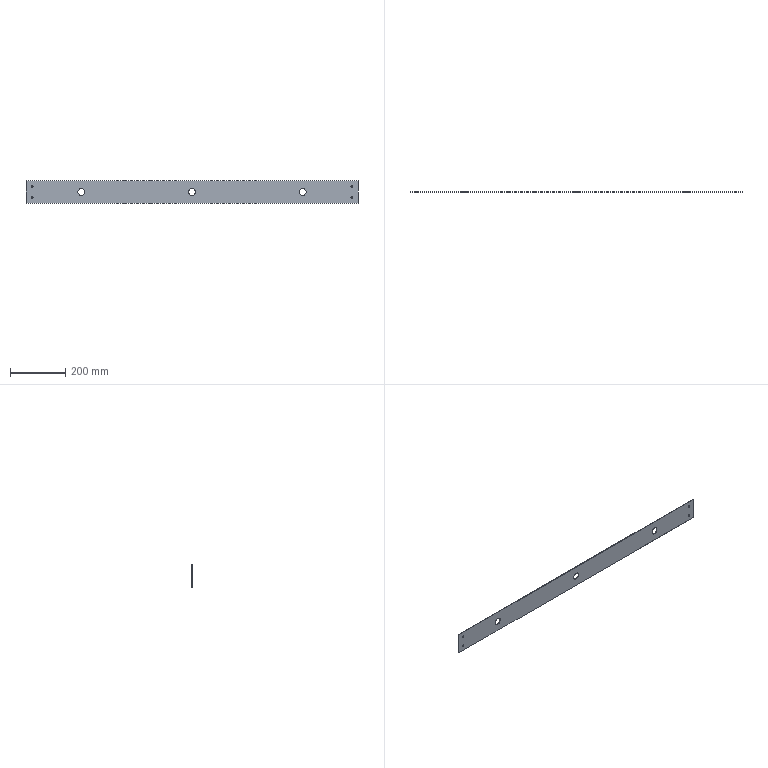Part | SolidWorks | features Extrusion 1 | 1 solid | 20 faces | box 1200 x 2 x 80 mm | volume 188829 mm3 | cylinder 14 | plane 6 | commonest cylinder face diameters 6 x8 25 x6
STEP:
#1=CARTESIAN_POINT('',(0.,2.,-12.5));
#2=VERTEX_POINT('',#1);
#3=CARTESIAN_POINT('',(0.,2.,12.5));
#4=VERTEX_POINT('',#3);
#5=CARTESIAN_POINT('',(0.,2.,0.));
#6=DIRECTION('',(0.,1.,0.));
#7=DIRECTION('',(0.,0.,1.));
#8=AXIS2_PLACEMENT_3D('',#5,#6,#7);
#9=CIRCLE('',#8,12.5);
#10=EDGE_CURVE('',#2,#4,#9,.T.);
#11=ORIENTED_EDGE('',*,*,#10,.T.);
#12=CARTESIAN_POINT('',(0.,0.,12.5));
#13=VERTEX_POINT('',#12);
#14=CARTESIAN_POINT('',(0.,2.,12.5));
#15=DIRECTION('',(0.,-1.,0.));
#16=VECTOR('',#15,1000.);
#17=LINE('',#14,#16);
#18=EDGE_CURVE('',#4,#13,#17,.T.);
#19=ORIENTED_EDGE('',*,*,#18,.T.);
#20=CARTESIAN_POINT('',(0.,0.,-12.5));
#21=VERTEX_POINT('',#20);
#22=CARTESIAN_POINT('',(0.,0.,0.));
#23=DIRECTION('',(0.,1.,0.));
#24=DIRECTION('',(0.,0.,1.));
#25=AXIS2_PLACEMENT_3D('',#22,#23,#24);
#26=CIRCLE('',#25,12.5);
#27=EDGE_CURVE('',#21,#13,#26,.T.);
#28=ORIENTED_EDGE('',*,*,#27,.F.);
#29=CARTESIAN_POINT('',(0.,2.,-12.5));
#30=DIRECTION('',(0.,-1.,0.));
#31=VECTOR('',#30,1000.);
#32=LINE('',#29,#31);
#33=EDGE_CURVE('',#2,#21,#32,.T.);
#34=ORIENTED_EDGE('',*,*,#33,.F.);
#35=EDGE_LOOP('',(#11,#19,#28,#34));
#36=FACE_OUTER_BOUND('',#35,.T.);
#37=CARTESIAN_POINT('',(0.,2.,0.));
#38=DIRECTION('',(0.,-1.,0.));
#39=DIRECTION('',(0.,0.,-1.));
#40=AXIS2_PLACEMENT_3D('',#37,#38,#39);
#41=CYLINDRICAL_SURFACE('',#40,12.5);
#42=ADVANCED_FACE('',(#36),#41,.F.);
#43=CARTESIAN_POINT('',(577.5,2.,17.));
#44=VERTEX_POINT('',#43);
#45=CARTESIAN_POINT('',(577.5,2.,23.));
#46=VERTEX_POINT('',#45);
#47=CARTESIAN_POINT('',(577.5,2.,20.));
#48=DIRECTION('',(0.,1.,0.));
#49=DIRECTION('',(0.,0.,1.));
#50=AXIS2_PLACEMENT_3D('',#47,#48,#49);
#51=CIRCLE('',#50,3.);
#52=EDGE_CURVE('',#44,#46,#51,.T.);
#53=ORIENTED_EDGE('',*,*,#52,.T.);
#54=CARTESIAN_POINT('',(577.5,0.,23.));
#55=VERTEX_POINT('',#54);
#56=CARTESIAN_POINT('',(577.5,2.,23.));
#57=DIRECTION('',(0.,-1.,0.));
#58=VECTOR('',#57,1000.);
#59=LINE('',#56,#58);
#60=EDGE_CURVE('',#46,#55,#59,.T.);
#61=ORIENTED_EDGE('',*,*,#60,.T.);
#62=CARTESIAN_POINT('',(577.5,0.,17.));
#63=VERTEX_POINT('',#62);
#64=CARTESIAN_POINT('',(577.5,0.,20.));
#65=DIRECTION('',(0.,1.,0.));
#66=DIRECTION('',(0.,0.,1.));
#67=AXIS2_PLACEMENT_3D('',#64,#65,#66);
#68=CIRCLE('',#67,3.);
#69=EDGE_CURVE('',#63,#55,#68,.T.);
#70=ORIENTED_EDGE('',*,*,#69,.F.);
#71=CARTESIAN_POINT('',(577.5,2.,17.));
#72=DIRECTION('',(0.,-1.,0.));
#73=VECTOR('',#72,1000.);
#74=LINE('',#71,#73);
#75=EDGE_CURVE('',#44,#63,#74,.T.);
#76=ORIENTED_EDGE('',*,*,#75,.F.);
#77=EDGE_LOOP('',(#53,#61,#70,#76));
#78=FACE_OUTER_BOUND('',#77,.T.);
#79=CARTESIAN_POINT('',(577.5,2.,20.));
#80=DIRECTION('',(0.,-1.,0.));
#81=DIRECTION('',(0.,0.,-1.));
#82=AXIS2_PLACEMENT_3D('',#79,#80,#81);
#83=CYLINDRICAL_SURFACE('',#82,3.);
#84=ADVANCED_FACE('',(#78),#83,.F.);
#85=CARTESIAN_POINT('',(-577.5,2.,17.));
#86=VERTEX_POINT('',#85);
#87=CARTESIAN_POINT('',(-577.5,2.,23.));
#88=VERTEX_POINT('',#87);
#89=CARTESIAN_POINT('',(-577.5,2.,20.));
#90=DIRECTION('',(0.,1.,0.));
#91=DIRECTION('',(0.,0.,1.));
#92=AXIS2_PLACEMENT_3D('',#89,#90,#91);
#93=CIRCLE('',#92,3.);
#94=EDGE_CURVE('',#86,#88,#93,.T.);
#95=ORIENTED_EDGE('',*,*,#94,.T.);
#96=CARTESIAN_POINT('',(-577.5,0.,23.));
#97=VERTEX_POINT('',#96);
#98=CARTESIAN_POINT('',(-577.5,2.,23.));
#99=DIRECTION('',(0.,-1.,0.));
#100=VECTOR('',#99,1000.);
#101=LINE('',#98,#100);
#102=EDGE_CURVE('',#88,#97,#101,.T.);
#103=ORIENTED_EDGE('',*,*,#102,.T.);
#104=CARTESIAN_POINT('',(-577.5,0.,17.));
#105=VERTEX_POINT('',#104);
#106=CARTESIAN_POINT('',(-577.5,0.,20.));
#107=DIRECTION('',(0.,1.,0.));
#108=DIRECTION('',(0.,0.,1.));
#109=AXIS2_PLACEMENT_3D('',#106,#107,#108);
#110=CIRCLE('',#109,3.);
#111=EDGE_CURVE('',#105,#97,#110,.T.);
#112=ORIENTED_EDGE('',*,*,#111,.F.);
#113=CARTESIAN_POINT('',(-577.5,2.,17.));
#114=DIRECTION('',(0.,-1.,0.));
#115=VECTOR('',#114,1000.);
#116=LINE('',#113,#115);
#117=EDGE_CURVE('',#86,#105,#116,.T.);
#118=ORIENTED_EDGE('',*,*,#117,.F.);
#119=EDGE_LOOP('',(#95,#103,#112,#118));
#120=FACE_OUTER_BOUND('',#119,.T.);
#121=CARTESIAN_POINT('',(-577.5,2.,20.));
#122=DIRECTION('',(0.,-1.,0.));
#123=DIRECTION('',(0.,0.,-1.));
#124=AXIS2_PLACEMENT_3D('',#121,#122,#123);
#125=CYLINDRICAL_SURFACE('',#124,3.);
#126=ADVANCED_FACE('',(#120),#125,.F.);
#127=CARTESIAN_POINT('',(-577.5,2.,-23.));
#128=VERTEX_POINT('',#127);
#129=CARTESIAN_POINT('',(-577.5,2.,-17.));
#130=VERTEX_POINT('',#129);
#131=CARTESIAN_POINT('',(-577.5,2.,-20.));
#132=DIRECTION('',(0.,1.,0.));
#133=DIRECTION('',(0.,0.,1.));
#134=AXIS2_PLACEMENT_3D('',#131,#132,#133);
#135=CIRCLE('',#134,3.);
#136=EDGE_CURVE('',#128,#130,#135,.T.);
#137=ORIENTED_EDGE('',*,*,#136,.T.);
#138=CARTESIAN_POINT('',(-577.5,0.,-17.));
#139=VERTEX_POINT('',#138);
#140=CARTESIAN_POINT('',(-577.5,2.,-17.));
#141=DIRECTION('',(0.,-1.,0.));
#142=VECTOR('',#141,1000.);
#143=LINE('',#140,#142);
#144=EDGE_CURVE('',#130,#139,#143,.T.);
#145=ORIENTED_EDGE('',*,*,#144,.T.);
#146=CARTESIAN_POINT('',(-577.5,0.,-23.));
#147=VERTEX_POINT('',#146);
#148=CARTESIAN_POINT('',(-577.5,0.,-20.));
#149=DIRECTION('',(0.,1.,0.));
#150=DIRECTION('',(0.,0.,1.));
#151=AXIS2_PLACEMENT_3D('',#148,#149,#150);
#152=CIRCLE('',#151,3.);
#153=EDGE_CURVE('',#147,#139,#152,.T.);
#154=ORIENTED_EDGE('',*,*,#153,.F.);
#155=CARTESIAN_POINT('',(-577.5,2.,-23.));
#156=DIRECTION('',(0.,-1.,0.));
#157=VECTOR('',#156,1000.);
#158=LINE('',#155,#157);
#159=EDGE_CURVE('',#128,#147,#158,.T.);
#160=ORIENTED_EDGE('',*,*,#159,.F.);
#161=EDGE_LOOP('',(#137,#145,#154,#160));
#162=FACE_OUTER_BOUND('',#161,.T.);
#163=CARTESIAN_POINT('',(-577.5,2.,-20.));
#164=DIRECTION('',(0.,-1.,0.));
#165=DIRECTION('',(0.,0.,-1.));
#166=AXIS2_PLACEMENT_3D('',#163,#164,#165);
#167=CYLINDRICAL_SURFACE('',#166,3.);
#168=ADVANCED_FACE('',(#162),#167,.F.);
#169=CARTESIAN_POINT('',(577.5,2.,-23.));
#170=VERTEX_POINT('',#169);
#171=CARTESIAN_POINT('',(577.5,2.,-17.));
#172=VERTEX_POINT('',#171);
#173=CARTESIAN_POINT('',(577.5,2.,-20.));
#174=DIRECTION('',(0.,1.,0.));
#175=DIRECTION('',(0.,0.,1.));
#176=AXIS2_PLACEMENT_3D('',#173,#174,#175);
#177=CIRCLE('',#176,3.);
#178=EDGE_CURVE('',#170,#172,#177,.T.);
#179=ORIENTED_EDGE('',*,*,#178,.T.);
#180=CARTESIAN_POINT('',(577.5,0.,-17.));
#181=VERTEX_POINT('',#180);
#182=CARTESIAN_POINT('',(577.5,2.,-17.));
#183=DIRECTION('',(0.,-1.,0.));
#184=VECTOR('',#183,1000.);
#185=LINE('',#182,#184);
#186=EDGE_CURVE('',#172,#181,#185,.T.);
#187=ORIENTED_EDGE('',*,*,#186,.T.);
#188=CARTESIAN_POINT('',(577.5,0.,-23.));
#189=VERTEX_POINT('',#188);
#190=CARTESIAN_POINT('',(577.5,0.,-20.));
#191=DIRECTION('',(0.,1.,0.));
#192=DIRECTION('',(0.,0.,1.));
#193=AXIS2_PLACEMENT_3D('',#190,#191,#192);
#194=CIRCLE('',#193,3.);
#195=EDGE_CURVE('',#189,#181,#194,.T.);
#196=ORIENTED_EDGE('',*,*,#195,.F.);
#197=CARTESIAN_POINT('',(577.5,2.,-23.));
#198=DIRECTION('',(0.,-1.,0.));
#199=VECTOR('',#198,1000.);
#200=LINE('',#197,#199);
#201=EDGE_CURVE('',#170,#189,#200,.T.);
#202=ORIENTED_EDGE('',*,*,#201,.F.);
#203=EDGE_LOOP('',(#179,#187,#196,#202));
#204=FACE_OUTER_BOUND('',#203,.T.);
#205=CARTESIAN_POINT('',(577.5,2.,-20.));
#206=DIRECTION('',(0.,-1.,0.));
#207=DIRECTION('',(0.,0.,-1.));
#208=AXIS2_PLACEMENT_3D('',#205,#206,#207);
#209=CYLINDRICAL_SURFACE('',#208,3.);
#210=ADVANCED_FACE('',(#204),#209,.F.);
#211=CARTESIAN_POINT('',(400.,2.,-12.5));
#212=VERTEX_POINT('',#211);
#213=CARTESIAN_POINT('',(400.,2.,12.5));
#214=VERTEX_POINT('',#213);
#215=CARTESIAN_POINT('',(400.,2.,0.));
#216=DIRECTION('',(0.,1.,0.));
#217=DIRECTION('',(0.,0.,1.));
#218=AXIS2_PLACEMENT_3D('',#215,#216,#217);
#219=CIRCLE('',#218,12.5);
#220=EDGE_CURVE('',#212,#214,#219,.T.);
#221=ORIENTED_EDGE('',*,*,#220,.T.);
#222=CARTESIAN_POINT('',(400.,0.,12.5));
#223=VERTEX_POINT('',#222);
#224=CARTESIAN_POINT('',(400.,2.,12.5));
#225=DIRECTION('',(0.,-1.,0.));
#226=VECTOR('',#225,1000.);
#227=LINE('',#224,#226);
#228=EDGE_CURVE('',#214,#223,#227,.T.);
#229=ORIENTED_EDGE('',*,*,#228,.T.);
#230=CARTESIAN_POINT('',(400.,0.,-12.5));
#231=VERTEX_POINT('',#230);
#232=CARTESIAN_POINT('',(400.,0.,0.));
#233=DIRECTION('',(0.,1.,0.));
#234=DIRECTION('',(0.,0.,1.));
#235=AXIS2_PLACEMENT_3D('',#232,#233,#234);
#236=CIRCLE('',#235,12.5);
#237=EDGE_CURVE('',#231,#223,#236,.T.);
#238=ORIENTED_EDGE('',*,*,#237,.F.);
#239=CARTESIAN_POINT('',(400.,2.,-12.5));
#240=DIRECTION('',(0.,-1.,0.));
#241=VECTOR('',#240,1000.);
#242=LINE('',#239,#241);
#243=EDGE_CURVE('',#212,#231,#242,.T.);
#244=ORIENTED_EDGE('',*,*,#243,.F.);
#245=EDGE_LOOP('',(#221,#229,#238,#244));
#246=FACE_OUTER_BOUND('',#245,.T.);
#247=CARTESIAN_POINT('',(400.,2.,0.));
#248=DIRECTION('',(0.,-1.,0.));
#249=DIRECTION('',(0.,0.,-1.));
#250=AXIS2_PLACEMENT_3D('',#247,#248,#249);
#251=CYLINDRICAL_SURFACE('',#250,12.5);
#252=ADVANCED_FACE('',(#246),#251,.F.);
#253=CARTESIAN_POINT('',(-400.,2.,-12.5));
#254=VERTEX_POINT('',#253);
#255=CARTESIAN_POINT('',(-400.,2.,12.5));
#256=VERTEX_POINT('',#255);
#257=CARTESIAN_POINT('',(-400.,2.,0.));
#258=DIRECTION('',(0.,1.,0.));
#259=DIRECTION('',(0.,0.,1.));
#260=AXIS2_PLACEMENT_3D('',#257,#258,#259);
#261=CIRCLE('',#260,12.5);
#262=EDGE_CURVE('',#254,#256,#261,.T.);
#263=ORIENTED_EDGE('',*,*,#262,.T.);
#264=CARTESIAN_POINT('',(-400.,0.,12.5));
#265=VERTEX_POINT('',#264);
#266=CARTESIAN_POINT('',(-400.,2.,12.5));
#267=DIRECTION('',(0.,-1.,0.));
#268=VECTOR('',#267,1000.);
#269=LINE('',#266,#268);
#270=EDGE_CURVE('',#256,#265,#269,.T.);
#271=ORIENTED_EDGE('',*,*,#270,.T.);
#272=CARTESIAN_POINT('',(-400.,0.,-12.5));
#273=VERTEX_POINT('',#272);
#274=CARTESIAN_POINT('',(-400.,0.,0.));
#275=DIRECTION('',(0.,1.,0.));
#276=DIRECTION('',(0.,0.,1.));
#277=AXIS2_PLACEMENT_3D('',#274,#275,#276);
#278=CIRCLE('',#277,12.5);
#279=EDGE_CURVE('',#273,#265,#278,.T.);
#280=ORIENTED_EDGE('',*,*,#279,.F.);
#281=CARTESIAN_POINT('',(-400.,2.,-12.5));
#282=DIRECTION('',(0.,-1.,0.));
#283=VECTOR('',#282,1000.);
#284=LINE('',#281,#283);
#285=EDGE_CURVE('',#254,#273,#284,.T.);
#286=ORIENTED_EDGE('',*,*,#285,.F.);
#287=EDGE_LOOP('',(#263,#271,#280,#286));
#288=FACE_OUTER_BOUND('',#287,.T.);
#289=CARTESIAN_POINT('',(-400.,2.,0.));
#290=DIRECTION('',(0.,-1.,0.));
#291=DIRECTION('',(0.,0.,-1.));
#292=AXIS2_PLACEMENT_3D('',#289,#290,#291);
#293=CYLINDRICAL_SURFACE('',#292,12.5);
#294=ADVANCED_FACE('',(#288),#293,.F.);
#295=ORIENTED_EDGE('',*,*,#52,.F.);
#296=CARTESIAN_POINT('',(577.5,2.,20.));
#297=DIRECTION('',(0.,1.,0.));
#298=DIRECTION('',(0.,0.,1.));
#299=AXIS2_PLACEMENT_3D('',#296,#297,#298);
#300=CIRCLE('',#299,3.);
#301=EDGE_CURVE('',#46,#44,#300,.T.);
#302=ORIENTED_EDGE('',*,*,#301,.F.);
#303=EDGE_LOOP('',(#295,#302));
#304=FACE_BOUND('',#303,.T.);
#305=ORIENTED_EDGE('',*,*,#136,.F.);
#306=CARTESIAN_POINT('',(-577.5,2.,-20.));
#307=DIRECTION('',(0.,1.,0.));
#308=DIRECTION('',(0.,0.,1.));
#309=AXIS2_PLACEMENT_3D('',#306,#307,#308);
#310=CIRCLE('',#309,3.);
#311=EDGE_CURVE('',#130,#128,#310,.T.);
#312=ORIENTED_EDGE('',*,*,#311,.F.);
#313=EDGE_LOOP('',(#305,#312));
#314=FACE_BOUND('',#313,.T.);
#315=ORIENTED_EDGE('',*,*,#220,.F.);
#316=CARTESIAN_POINT('',(400.,2.,0.));
#317=DIRECTION('',(0.,1.,0.));
#318=DIRECTION('',(0.,0.,1.));
#319=AXIS2_PLACEMENT_3D('',#316,#317,#318);
#320=CIRCLE('',#319,12.5);
#321=EDGE_CURVE('',#214,#212,#320,.T.);
#322=ORIENTED_EDGE('',*,*,#321,.F.);
#323=EDGE_LOOP('',(#315,#322));
#324=FACE_BOUND('',#323,.T.);
#325=CARTESIAN_POINT('',(-600.,2.,-40.));
#326=VERTEX_POINT('',#325);
#327=CARTESIAN_POINT('',(-600.,2.,40.));
#328=VERTEX_POINT('',#327);
#329=CARTESIAN_POINT('',(-600.,2.,40.));
#330=DIRECTION('',(0.,0.,1.));
#331=VECTOR('',#330,1000.);
#332=LINE('',#329,#331);
#333=EDGE_CURVE('',#326,#328,#332,.T.);
#334=ORIENTED_EDGE('',*,*,#333,.T.);
#335=CARTESIAN_POINT('',(600.,2.,40.));
#336=VERTEX_POINT('',#335);
#337=CARTESIAN_POINT('',(600.,2.,40.));
#338=DIRECTION('',(1.,0.,0.));
#339=VECTOR('',#338,1000.);
#340=LINE('',#337,#339);
#341=EDGE_CURVE('',#328,#336,#340,.T.);
#342=ORIENTED_EDGE('',*,*,#341,.T.);
#343=CARTESIAN_POINT('',(600.,2.,-40.));
#344=VERTEX_POINT('',#343);
#345=CARTESIAN_POINT('',(600.,2.,40.));
#346=DIRECTION('',(0.,0.,-1.));
#347=VECTOR('',#346,1000.);
#348=LINE('',#345,#347);
#349=EDGE_CURVE('',#336,#344,#348,.T.);
#350=ORIENTED_EDGE('',*,*,#349,.T.);
#351=CARTESIAN_POINT('',(600.,2.,-40.));
#352=DIRECTION('',(-1.,0.,0.));
#353=VECTOR('',#352,1000.);
#354=LINE('',#351,#353);
#355=EDGE_CURVE('',#344,#326,#354,.T.);
#356=ORIENTED_EDGE('',*,*,#355,.T.);
#357=EDGE_LOOP('',(#334,#342,#350,#356));
#358=FACE_OUTER_BOUND('',#357,.T.);
#359=ORIENTED_EDGE('',*,*,#262,.F.);
#360=CARTESIAN_POINT('',(-400.,2.,0.));
#361=DIRECTION('',(0.,1.,0.));
#362=DIRECTION('',(0.,0.,1.));
#363=AXIS2_PLACEMENT_3D('',#360,#361,#362);
#364=CIRCLE('',#363,12.5);
#365=EDGE_CURVE('',#256,#254,#364,.T.);
#366=ORIENTED_EDGE('',*,*,#365,.F.);
#367=EDGE_LOOP('',(#359,#366));
#368=FACE_BOUND('',#367,.T.);
#369=ORIENTED_EDGE('',*,*,#178,.F.);
#370=CARTESIAN_POINT('',(577.5,2.,-20.));
#371=DIRECTION('',(0.,1.,0.));
#372=DIRECTION('',(0.,0.,1.));
#373=AXIS2_PLACEMENT_3D('',#370,#371,#372);
#374=CIRCLE('',#373,3.);
#375=EDGE_CURVE('',#172,#170,#374,.T.);
#376=ORIENTED_EDGE('',*,*,#375,.F.);
#377=EDGE_LOOP('',(#369,#376));
#378=FACE_BOUND('',#377,.T.);
#379=ORIENTED_EDGE('',*,*,#94,.F.);
#380=CARTESIAN_POINT('',(-577.5,2.,20.));
#381=DIRECTION('',(0.,1.,0.));
#382=DIRECTION('',(0.,0.,1.));
#383=AXIS2_PLACEMENT_3D('',#380,#381,#382);
#384=CIRCLE('',#383,3.);
#385=EDGE_CURVE('',#88,#86,#384,.T.);
#386=ORIENTED_EDGE('',*,*,#385,.F.);
#387=EDGE_LOOP('',(#379,#386));
#388=FACE_BOUND('',#387,.T.);
#389=ORIENTED_EDGE('',*,*,#10,.F.);
#390=CARTESIAN_POINT('',(0.,2.,0.));
#391=DIRECTION('',(0.,1.,0.));
#392=DIRECTION('',(0.,0.,1.));
#393=AXIS2_PLACEMENT_3D('',#390,#391,#392);
#394=CIRCLE('',#393,12.5);
#395=EDGE_CURVE('',#4,#2,#394,.T.);
#396=ORIENTED_EDGE('',*,*,#395,.F.);
#397=EDGE_LOOP('',(#389,#396));
#398=FACE_BOUND('',#397,.T.);
#399=CARTESIAN_POINT('',(0.,2.,0.));
#400=DIRECTION('',(0.,1.,0.));
#401=DIRECTION('',(0.,0.,1.));
#402=AXIS2_PLACEMENT_3D('',#399,#400,#401);
#403=PLANE('',#402);
#404=ADVANCED_FACE('',(#304,#314,#324,#358,#368,#378,#388,#398),#403,.T.);
#405=CARTESIAN_POINT('',(-600.,0.,-40.));
#406=VERTEX_POINT('',#405);
#407=CARTESIAN_POINT('',(-600.,0.,40.));
#408=VERTEX_POINT('',#407);
#409=CARTESIAN_POINT('',(-600.,0.,40.));
#410=DIRECTION('',(0.,0.,1.));
#411=VECTOR('',#410,1000.);
#412=LINE('',#409,#411);
#413=EDGE_CURVE('',#406,#408,#412,.T.);
#414=ORIENTED_EDGE('',*,*,#413,.F.);
#415=CARTESIAN_POINT('',(600.,0.,-40.));
#416=VERTEX_POINT('',#415);
#417=CARTESIAN_POINT('',(600.,0.,-40.));
#418=DIRECTION('',(-1.,0.,0.));
#419=VECTOR('',#418,1000.);
#420=LINE('',#417,#419);
#421=EDGE_CURVE('',#416,#406,#420,.T.);
#422=ORIENTED_EDGE('',*,*,#421,.F.);
#423=CARTESIAN_POINT('',(600.,0.,40.));
#424=VERTEX_POINT('',#423);
#425=CARTESIAN_POINT('',(600.,0.,40.));
#426=DIRECTION('',(0.,0.,-1.));
#427=VECTOR('',#426,1000.);
#428=LINE('',#425,#427);
#429=EDGE_CURVE('',#424,#416,#428,.T.);
#430=ORIENTED_EDGE('',*,*,#429,.F.);
#431=CARTESIAN_POINT('',(600.,0.,40.));
#432=DIRECTION('',(1.,0.,0.));
#433=VECTOR('',#432,1000.);
#434=LINE('',#431,#433);
#435=EDGE_CURVE('',#408,#424,#434,.T.);
#436=ORIENTED_EDGE('',*,*,#435,.F.);
#437=EDGE_LOOP('',(#414,#422,#430,#436));
#438=FACE_OUTER_BOUND('',#437,.T.);
#439=ORIENTED_EDGE('',*,*,#279,.T.);
#440=CARTESIAN_POINT('',(-400.,0.,0.));
#441=DIRECTION('',(0.,1.,0.));
#442=DIRECTION('',(0.,0.,1.));
#443=AXIS2_PLACEMENT_3D('',#440,#441,#442);
#444=CIRCLE('',#443,12.5);
#445=EDGE_CURVE('',#265,#273,#444,.T.);
#446=ORIENTED_EDGE('',*,*,#445,.T.);
#447=EDGE_LOOP('',(#439,#446));
#448=FACE_BOUND('',#447,.T.);
#449=ORIENTED_EDGE('',*,*,#237,.T.);
#450=CARTESIAN_POINT('',(400.,0.,0.));
#451=DIRECTION('',(0.,1.,0.));
#452=DIRECTION('',(0.,0.,1.));
#453=AXIS2_PLACEMENT_3D('',#450,#451,#452);
#454=CIRCLE('',#453,12.5);
#455=EDGE_CURVE('',#223,#231,#454,.T.);
#456=ORIENTED_EDGE('',*,*,#455,.T.);
#457=EDGE_LOOP('',(#449,#456));
#458=FACE_BOUND('',#457,.T.);
#459=ORIENTED_EDGE('',*,*,#195,.T.);
#460=CARTESIAN_POINT('',(577.5,0.,-20.));
#461=DIRECTION('',(0.,1.,0.));
#462=DIRECTION('',(0.,0.,1.));
#463=AXIS2_PLACEMENT_3D('',#460,#461,#462);
#464=CIRCLE('',#463,3.);
#465=EDGE_CURVE('',#181,#189,#464,.T.);
#466=ORIENTED_EDGE('',*,*,#465,.T.);
#467=EDGE_LOOP('',(#459,#466));
#468=FACE_BOUND('',#467,.T.);
#469=ORIENTED_EDGE('',*,*,#153,.T.);
#470=CARTESIAN_POINT('',(-577.5,0.,-20.));
#471=DIRECTION('',(0.,1.,0.));
#472=DIRECTION('',(0.,0.,1.));
#473=AXIS2_PLACEMENT_3D('',#470,#471,#472);
#474=CIRCLE('',#473,3.);
#475=EDGE_CURVE('',#139,#147,#474,.T.);
#476=ORIENTED_EDGE('',*,*,#475,.T.);
#477=EDGE_LOOP('',(#469,#476));
#478=FACE_BOUND('',#477,.T.);
#479=ORIENTED_EDGE('',*,*,#111,.T.);
#480=CARTESIAN_POINT('',(-577.5,0.,20.));
#481=DIRECTION('',(0.,1.,0.));
#482=DIRECTION('',(0.,0.,1.));
#483=AXIS2_PLACEMENT_3D('',#480,#481,#482);
#484=CIRCLE('',#483,3.);
#485=EDGE_CURVE('',#97,#105,#484,.T.);
#486=ORIENTED_EDGE('',*,*,#485,.T.);
#487=EDGE_LOOP('',(#479,#486));
#488=FACE_BOUND('',#487,.T.);
#489=ORIENTED_EDGE('',*,*,#69,.T.);
#490=CARTESIAN_POINT('',(577.5,0.,20.));
#491=DIRECTION('',(0.,1.,0.));
#492=DIRECTION('',(0.,0.,1.));
#493=AXIS2_PLACEMENT_3D('',#490,#491,#492);
#494=CIRCLE('',#493,3.);
#495=EDGE_CURVE('',#55,#63,#494,.T.);
#496=ORIENTED_EDGE('',*,*,#495,.T.);
#497=EDGE_LOOP('',(#489,#496));
#498=FACE_BOUND('',#497,.T.);
#499=ORIENTED_EDGE('',*,*,#27,.T.);
#500=CARTESIAN_POINT('',(0.,0.,0.));
#501=DIRECTION('',(0.,1.,0.));
#502=DIRECTION('',(0.,0.,1.));
#503=AXIS2_PLACEMENT_3D('',#500,#501,#502);
#504=CIRCLE('',#503,12.5);
#505=EDGE_CURVE('',#13,#21,#504,.T.);
#506=ORIENTED_EDGE('',*,*,#505,.T.);
#507=EDGE_LOOP('',(#499,#506));
#508=FACE_BOUND('',#507,.T.);
#509=CARTESIAN_POINT('',(0.,0.,0.));
#510=DIRECTION('',(0.,1.,0.));
#511=DIRECTION('',(0.,0.,1.));
#512=AXIS2_PLACEMENT_3D('',#509,#510,#511);
#513=PLANE('',#512);
#514=ADVANCED_FACE('',(#438,#448,#458,#468,#478,#488,#498,#508),#513,.F.);
#515=ORIENTED_EDGE('',*,*,#413,.T.);
#516=CARTESIAN_POINT('',(-600.,2.,40.));
#517=DIRECTION('',(0.,-1.,0.));
#518=VECTOR('',#517,1000.);
#519=LINE('',#516,#518);
#520=EDGE_CURVE('',#328,#408,#519,.T.);
#521=ORIENTED_EDGE('',*,*,#520,.F.);
#522=ORIENTED_EDGE('',*,*,#333,.F.);
#523=CARTESIAN_POINT('',(-600.,2.,-40.));
#524=DIRECTION('',(0.,-1.,0.));
#525=VECTOR('',#524,1000.);
#526=LINE('',#523,#525);
#527=EDGE_CURVE('',#326,#406,#526,.T.);
#528=ORIENTED_EDGE('',*,*,#527,.T.);
#529=EDGE_LOOP('',(#515,#521,#522,#528));
#530=FACE_OUTER_BOUND('',#529,.T.);
#531=CARTESIAN_POINT('',(-600.,2.,40.));
#532=DIRECTION('',(1.,0.,0.));
#533=DIRECTION('',(0.,0.,-1.));
#534=AXIS2_PLACEMENT_3D('',#531,#532,#533);
#535=PLANE('',#534);
#536=ADVANCED_FACE('',(#530),#535,.F.);
#537=ORIENTED_EDGE('',*,*,#435,.T.);
#538=CARTESIAN_POINT('',(600.,2.,40.));
#539=DIRECTION('',(0.,-1.,0.));
#540=VECTOR('',#539,1000.);
#541=LINE('',#538,#540);
#542=EDGE_CURVE('',#336,#424,#541,.T.);
#543=ORIENTED_EDGE('',*,*,#542,.F.);
#544=ORIENTED_EDGE('',*,*,#341,.F.);
#545=ORIENTED_EDGE('',*,*,#520,.T.);
#546=EDGE_LOOP('',(#537,#543,#544,#545));
#547=FACE_OUTER_BOUND('',#546,.T.);
#548=CARTESIAN_POINT('',(600.,2.,40.));
#549=DIRECTION('',(0.,0.,-1.));
#550=DIRECTION('',(-1.,0.,0.));
#551=AXIS2_PLACEMENT_3D('',#548,#549,#550);
#552=PLANE('',#551);
#553=ADVANCED_FACE('',(#547),#552,.F.);
#554=ORIENTED_EDGE('',*,*,#429,.T.);
#555=CARTESIAN_POINT('',(600.,2.,-40.));
#556=DIRECTION('',(0.,-1.,0.));
#557=VECTOR('',#556,1000.);
#558=LINE('',#555,#557);
#559=EDGE_CURVE('',#344,#416,#558,.T.);
#560=ORIENTED_EDGE('',*,*,#559,.F.);
#561=ORIENTED_EDGE('',*,*,#349,.F.);
#562=ORIENTED_EDGE('',*,*,#542,.T.);
#563=EDGE_LOOP('',(#554,#560,#561,#562));
#564=FACE_OUTER_BOUND('',#563,.T.);
#565=CARTESIAN_POINT('',(600.,2.,40.));
#566=DIRECTION('',(-1.,0.,0.));
#567=DIRECTION('',(0.,0.,1.));
#568=AXIS2_PLACEMENT_3D('',#565,#566,#567);
#569=PLANE('',#568);
#570=ADVANCED_FACE('',(#564),#569,.F.);
#571=ORIENTED_EDGE('',*,*,#421,.T.);
#572=ORIENTED_EDGE('',*,*,#527,.F.);
#573=ORIENTED_EDGE('',*,*,#355,.F.);
#574=ORIENTED_EDGE('',*,*,#559,.T.);
#575=EDGE_LOOP('',(#571,#572,#573,#574));
#576=FACE_OUTER_BOUND('',#575,.T.);
#577=CARTESIAN_POINT('',(600.,2.,-40.));
#578=DIRECTION('',(0.,0.,1.));
#579=DIRECTION('',(1.,0.,0.));
#580=AXIS2_PLACEMENT_3D('',#577,#578,#579);
#581=PLANE('',#580);
#582=ADVANCED_FACE('',(#576),#581,.F.);
#583=ORIENTED_EDGE('',*,*,#270,.F.);
#584=ORIENTED_EDGE('',*,*,#365,.T.);
#585=ORIENTED_EDGE('',*,*,#285,.T.);
#586=ORIENTED_EDGE('',*,*,#445,.F.);
#587=EDGE_LOOP('',(#583,#584,#585,#586));
#588=FACE_OUTER_BOUND('',#587,.T.);
#589=CARTESIAN_POINT('',(-400.,2.,0.));
#590=DIRECTION('',(0.,-1.,0.));
#591=DIRECTION('',(0.,0.,-1.));
#592=AXIS2_PLACEMENT_3D('',#589,#590,#591);
#593=CYLINDRICAL_SURFACE('',#592,12.5);
#594=ADVANCED_FACE('',(#588),#593,.F.);
#595=ORIENTED_EDGE('',*,*,#228,.F.);
#596=ORIENTED_EDGE('',*,*,#321,.T.);
#597=ORIENTED_EDGE('',*,*,#243,.T.);
#598=ORIENTED_EDGE('',*,*,#455,.F.);
#599=EDGE_LOOP('',(#595,#596,#597,#598));
#600=FACE_OUTER_BOUND('',#599,.T.);
#601=CARTESIAN_POINT('',(400.,2.,0.));
#602=DIRECTION('',(0.,-1.,0.));
#603=DIRECTION('',(0.,0.,-1.));
#604=AXIS2_PLACEMENT_3D('',#601,#602,#603);
#605=CYLINDRICAL_SURFACE('',#604,12.5);
#606=ADVANCED_FACE('',(#600),#605,.F.);
#607=ORIENTED_EDGE('',*,*,#186,.F.);
#608=ORIENTED_EDGE('',*,*,#375,.T.);
#609=ORIENTED_EDGE('',*,*,#201,.T.);
#610=ORIENTED_EDGE('',*,*,#465,.F.);
#611=EDGE_LOOP('',(#607,#608,#609,#610));
#612=FACE_OUTER_BOUND('',#611,.T.);
#613=CARTESIAN_POINT('',(577.5,2.,-20.));
#614=DIRECTION('',(0.,-1.,0.));
#615=DIRECTION('',(0.,0.,-1.));
#616=AXIS2_PLACEMENT_3D('',#613,#614,#615);
#617=CYLINDRICAL_SURFACE('',#616,3.);
#618=ADVANCED_FACE('',(#612),#617,.F.);
#619=ORIENTED_EDGE('',*,*,#144,.F.);
#620=ORIENTED_EDGE('',*,*,#311,.T.);
#621=ORIENTED_EDGE('',*,*,#159,.T.);
#622=ORIENTED_EDGE('',*,*,#475,.F.);
#623=EDGE_LOOP('',(#619,#620,#621,#622));
#624=FACE_OUTER_BOUND('',#623,.T.);
#625=CARTESIAN_POINT('',(-577.5,2.,-20.));
#626=DIRECTION('',(0.,-1.,0.));
#627=DIRECTION('',(0.,0.,-1.));
#628=AXIS2_PLACEMENT_3D('',#625,#626,#627);
#629=CYLINDRICAL_SURFACE('',#628,3.);
#630=ADVANCED_FACE('',(#624),#629,.F.);
#631=ORIENTED_EDGE('',*,*,#102,.F.);
#632=ORIENTED_EDGE('',*,*,#385,.T.);
#633=ORIENTED_EDGE('',*,*,#117,.T.);
#634=ORIENTED_EDGE('',*,*,#485,.F.);
#635=EDGE_LOOP('',(#631,#632,#633,#634));
#636=FACE_OUTER_BOUND('',#635,.T.);
#637=CARTESIAN_POINT('',(-577.5,2.,20.));
#638=DIRECTION('',(0.,-1.,0.));
#639=DIRECTION('',(0.,0.,-1.));
#640=AXIS2_PLACEMENT_3D('',#637,#638,#639);
#641=CYLINDRICAL_SURFACE('',#640,3.);
#642=ADVANCED_FACE('',(#636),#641,.F.);
#643=ORIENTED_EDGE('',*,*,#60,.F.);
#644=ORIENTED_EDGE('',*,*,#301,.T.);
#645=ORIENTED_EDGE('',*,*,#75,.T.);
#646=ORIENTED_EDGE('',*,*,#495,.F.);
#647=EDGE_LOOP('',(#643,#644,#645,#646));
#648=FACE_OUTER_BOUND('',#647,.T.);
#649=CARTESIAN_POINT('',(577.5,2.,20.));
#650=DIRECTION('',(0.,-1.,0.));
#651=DIRECTION('',(0.,0.,-1.));
#652=AXIS2_PLACEMENT_3D('',#649,#650,#651);
#653=CYLINDRICAL_SURFACE('',#652,3.);
#654=ADVANCED_FACE('',(#648),#653,.F.);
#655=ORIENTED_EDGE('',*,*,#18,.F.);
#656=ORIENTED_EDGE('',*,*,#395,.T.);
#657=ORIENTED_EDGE('',*,*,#33,.T.);
#658=ORIENTED_EDGE('',*,*,#505,.F.);
#659=EDGE_LOOP('',(#655,#656,#657,#658));
#660=FACE_OUTER_BOUND('',#659,.T.);
#661=CARTESIAN_POINT('',(0.,2.,0.));
#662=DIRECTION('',(0.,-1.,0.));
#663=DIRECTION('',(0.,0.,-1.));
#664=AXIS2_PLACEMENT_3D('',#661,#662,#663);
#665=CYLINDRICAL_SURFACE('',#664,12.5);
#666=ADVANCED_FACE('',(#660),#665,.F.);
#667=CLOSED_SHELL('',(#42,#84,#126,#168,#210,#252,#294,#404,#514,#536,#553,#570,#582,#594,#606,#618,#630,#642,#654,#666));
#668=MANIFOLD_SOLID_BREP('',#667);
#669=CARTESIAN_POINT('',(0.,0.,0.));
#670=DIRECTION('',(0.,0.,1.));
#671=DIRECTION('',(1.,0.,0.));
#672=AXIS2_PLACEMENT_3D('',#669,#670,#671);
#673=(LENGTH_UNIT()NAMED_UNIT(*)SI_UNIT(.MILLI.,.METRE.));
#674=UNCERTAINTY_MEASURE_WITH_UNIT(LENGTH_MEASURE(0.00001),#673,'','');
#675=(NAMED_UNIT(*)PLANE_ANGLE_UNIT()SI_UNIT($,.RADIAN.));
#676=(NAMED_UNIT(*)SI_UNIT($,.STERADIAN.)SOLID_ANGLE_UNIT());
#677=(GEOMETRIC_REPRESENTATION_CONTEXT(3)GLOBAL_UNCERTAINTY_ASSIGNED_CONTEXT((#674))GLOBAL_UNIT_ASSIGNED_CONTEXT((#673,#675,#676))REPRESENTATION_CONTEXT('',''));
#678=ADVANCED_BREP_SHAPE_REPRESENTATION('',(#668,#672),#677);